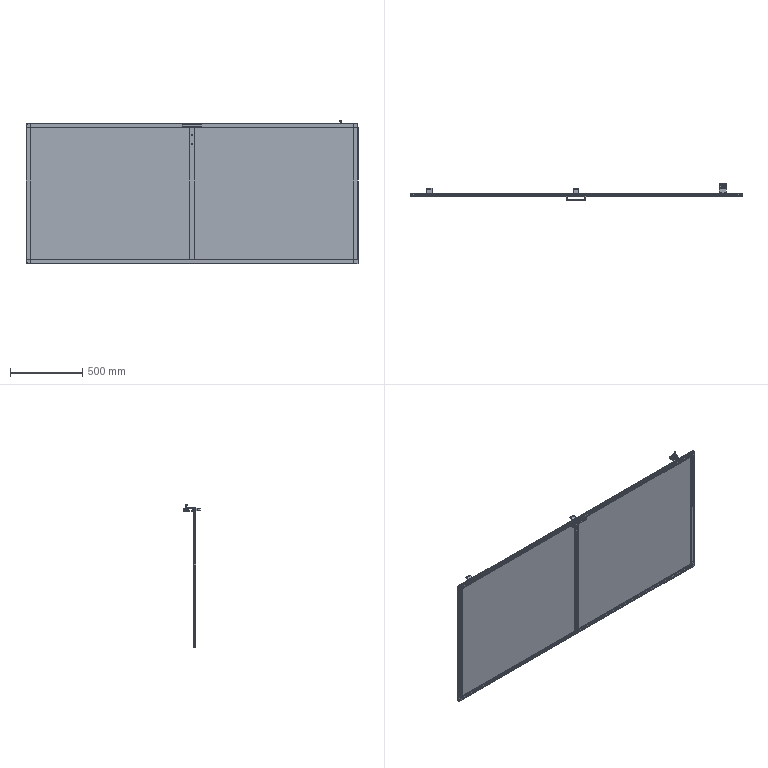Part | SolidWorks | features LocalLPattern 3, ReferencePattern 2, CompositeCurve 1 | 50 solids | 2518 faces | box 2296 x 114.543 x 991.55 mm | volume 12200814 mm3 | plane 1227 | cylinder 670 | cone 394 | spline 128 | torus 87 | sphere 12 | commonest cylinder face diameters 5 x103 1 x83 4.5 x64 11 x52 7 x32 4 x29